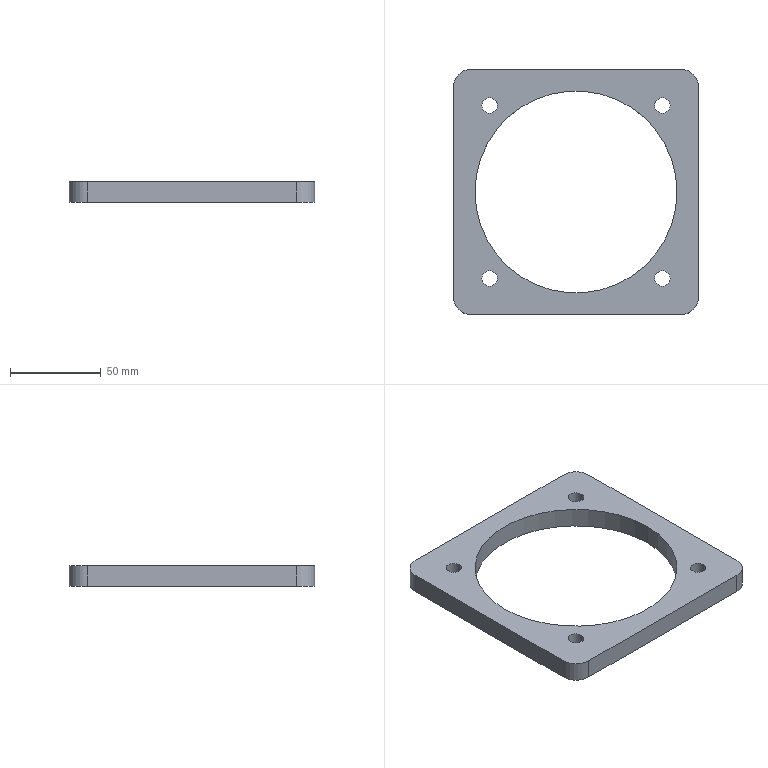Part | SolidWorks | features FlatPattern 1, HoleWzd 1, SMBaseFlange 1, SheetMetal 1 | 1 solid | 20 faces | box 135 x 135 x 11 mm | volume 90588 mm3 | cylinder 14 | plane 6 | commonest cylinder face diameters 8.5 x8 20 x4 111 x2
STEP:
#1=CARTESIAN_POINT('',(-51.75,47.5,-11.));
#2=VERTEX_POINT('',#1);
#3=CARTESIAN_POINT('',(-43.25,47.5,-11.));
#4=VERTEX_POINT('',#3);
#5=CARTESIAN_POINT('',(-47.5,47.5,-11.));
#6=DIRECTION('',(0.,0.,1.));
#7=DIRECTION('',(1.,0.,0.));
#8=AXIS2_PLACEMENT_3D('',#5,#6,#7);
#9=CIRCLE('',#8,4.25);
#10=EDGE_CURVE('',#2,#4,#9,.T.);
#11=ORIENTED_EDGE('',*,*,#10,.F.);
#12=CARTESIAN_POINT('',(-51.75,47.5,0.));
#13=VERTEX_POINT('',#12);
#14=CARTESIAN_POINT('',(-51.75,47.5,0.));
#15=DIRECTION('',(0.,0.,1.));
#16=VECTOR('',#15,1000.);
#17=LINE('',#14,#16);
#18=EDGE_CURVE('',#2,#13,#17,.T.);
#19=ORIENTED_EDGE('',*,*,#18,.T.);
#20=CARTESIAN_POINT('',(-43.25,47.5,0.));
#21=VERTEX_POINT('',#20);
#22=CARTESIAN_POINT('',(-47.5,47.5,0.));
#23=DIRECTION('',(0.,0.,1.));
#24=DIRECTION('',(1.,0.,0.));
#25=AXIS2_PLACEMENT_3D('',#22,#23,#24);
#26=CIRCLE('',#25,4.25);
#27=EDGE_CURVE('',#13,#21,#26,.T.);
#28=ORIENTED_EDGE('',*,*,#27,.T.);
#29=CARTESIAN_POINT('',(-43.25,47.5,0.));
#30=DIRECTION('',(0.,0.,1.));
#31=VECTOR('',#30,1000.);
#32=LINE('',#29,#31);
#33=EDGE_CURVE('',#4,#21,#32,.T.);
#34=ORIENTED_EDGE('',*,*,#33,.F.);
#35=EDGE_LOOP('',(#11,#19,#28,#34));
#36=FACE_OUTER_BOUND('',#35,.T.);
#37=CARTESIAN_POINT('',(-47.5,47.5,0.));
#38=DIRECTION('',(0.,0.,1.));
#39=DIRECTION('',(1.,0.,0.));
#40=AXIS2_PLACEMENT_3D('',#37,#38,#39);
#41=CYLINDRICAL_SURFACE('',#40,4.25);
#42=ADVANCED_FACE('',(#36),#41,.F.);
#43=CARTESIAN_POINT('',(43.25,47.5,-11.));
#44=VERTEX_POINT('',#43);
#45=CARTESIAN_POINT('',(51.75,47.5,-11.));
#46=VERTEX_POINT('',#45);
#47=CARTESIAN_POINT('',(47.5,47.5,-11.));
#48=DIRECTION('',(0.,0.,1.));
#49=DIRECTION('',(1.,0.,0.));
#50=AXIS2_PLACEMENT_3D('',#47,#48,#49);
#51=CIRCLE('',#50,4.25);
#52=EDGE_CURVE('',#44,#46,#51,.T.);
#53=ORIENTED_EDGE('',*,*,#52,.F.);
#54=CARTESIAN_POINT('',(43.25,47.5,0.));
#55=VERTEX_POINT('',#54);
#56=CARTESIAN_POINT('',(43.25,47.5,0.));
#57=DIRECTION('',(0.,0.,1.));
#58=VECTOR('',#57,1000.);
#59=LINE('',#56,#58);
#60=EDGE_CURVE('',#44,#55,#59,.T.);
#61=ORIENTED_EDGE('',*,*,#60,.T.);
#62=CARTESIAN_POINT('',(51.75,47.5,0.));
#63=VERTEX_POINT('',#62);
#64=CARTESIAN_POINT('',(47.5,47.5,0.));
#65=DIRECTION('',(0.,0.,1.));
#66=DIRECTION('',(1.,0.,0.));
#67=AXIS2_PLACEMENT_3D('',#64,#65,#66);
#68=CIRCLE('',#67,4.25);
#69=EDGE_CURVE('',#55,#63,#68,.T.);
#70=ORIENTED_EDGE('',*,*,#69,.T.);
#71=CARTESIAN_POINT('',(51.75,47.5,0.));
#72=DIRECTION('',(0.,0.,1.));
#73=VECTOR('',#72,1000.);
#74=LINE('',#71,#73);
#75=EDGE_CURVE('',#46,#63,#74,.T.);
#76=ORIENTED_EDGE('',*,*,#75,.F.);
#77=EDGE_LOOP('',(#53,#61,#70,#76));
#78=FACE_OUTER_BOUND('',#77,.T.);
#79=CARTESIAN_POINT('',(47.5,47.5,0.));
#80=DIRECTION('',(0.,0.,1.));
#81=DIRECTION('',(1.,0.,0.));
#82=AXIS2_PLACEMENT_3D('',#79,#80,#81);
#83=CYLINDRICAL_SURFACE('',#82,4.25);
#84=ADVANCED_FACE('',(#78),#83,.F.);
#85=CARTESIAN_POINT('',(43.25,-47.5,-11.));
#86=VERTEX_POINT('',#85);
#87=CARTESIAN_POINT('',(51.75,-47.5,-11.));
#88=VERTEX_POINT('',#87);
#89=CARTESIAN_POINT('',(47.5,-47.5,-11.));
#90=DIRECTION('',(0.,0.,1.));
#91=DIRECTION('',(1.,0.,0.));
#92=AXIS2_PLACEMENT_3D('',#89,#90,#91);
#93=CIRCLE('',#92,4.25);
#94=EDGE_CURVE('',#86,#88,#93,.T.);
#95=ORIENTED_EDGE('',*,*,#94,.F.);
#96=CARTESIAN_POINT('',(43.25,-47.5,0.));
#97=VERTEX_POINT('',#96);
#98=CARTESIAN_POINT('',(43.25,-47.5,0.));
#99=DIRECTION('',(0.,0.,1.));
#100=VECTOR('',#99,1000.);
#101=LINE('',#98,#100);
#102=EDGE_CURVE('',#86,#97,#101,.T.);
#103=ORIENTED_EDGE('',*,*,#102,.T.);
#104=CARTESIAN_POINT('',(51.75,-47.5,0.));
#105=VERTEX_POINT('',#104);
#106=CARTESIAN_POINT('',(47.5,-47.5,0.));
#107=DIRECTION('',(0.,0.,1.));
#108=DIRECTION('',(1.,0.,0.));
#109=AXIS2_PLACEMENT_3D('',#106,#107,#108);
#110=CIRCLE('',#109,4.25);
#111=EDGE_CURVE('',#97,#105,#110,.T.);
#112=ORIENTED_EDGE('',*,*,#111,.T.);
#113=CARTESIAN_POINT('',(51.75,-47.5,0.));
#114=DIRECTION('',(0.,0.,1.));
#115=VECTOR('',#114,1000.);
#116=LINE('',#113,#115);
#117=EDGE_CURVE('',#88,#105,#116,.T.);
#118=ORIENTED_EDGE('',*,*,#117,.F.);
#119=EDGE_LOOP('',(#95,#103,#112,#118));
#120=FACE_OUTER_BOUND('',#119,.T.);
#121=CARTESIAN_POINT('',(47.5,-47.5,0.));
#122=DIRECTION('',(0.,0.,1.));
#123=DIRECTION('',(1.,0.,0.));
#124=AXIS2_PLACEMENT_3D('',#121,#122,#123);
#125=CYLINDRICAL_SURFACE('',#124,4.25);
#126=ADVANCED_FACE('',(#120),#125,.F.);
#127=CARTESIAN_POINT('',(-51.75,-47.5,-11.));
#128=VERTEX_POINT('',#127);
#129=CARTESIAN_POINT('',(-43.25,-47.5,-11.));
#130=VERTEX_POINT('',#129);
#131=CARTESIAN_POINT('',(-47.5,-47.5,-11.));
#132=DIRECTION('',(0.,0.,1.));
#133=DIRECTION('',(1.,0.,0.));
#134=AXIS2_PLACEMENT_3D('',#131,#132,#133);
#135=CIRCLE('',#134,4.25);
#136=EDGE_CURVE('',#128,#130,#135,.T.);
#137=ORIENTED_EDGE('',*,*,#136,.F.);
#138=CARTESIAN_POINT('',(-51.75,-47.5,0.));
#139=VERTEX_POINT('',#138);
#140=CARTESIAN_POINT('',(-51.75,-47.5,0.));
#141=DIRECTION('',(0.,0.,1.));
#142=VECTOR('',#141,1000.);
#143=LINE('',#140,#142);
#144=EDGE_CURVE('',#128,#139,#143,.T.);
#145=ORIENTED_EDGE('',*,*,#144,.T.);
#146=CARTESIAN_POINT('',(-43.25,-47.5,0.));
#147=VERTEX_POINT('',#146);
#148=CARTESIAN_POINT('',(-47.5,-47.5,0.));
#149=DIRECTION('',(0.,0.,1.));
#150=DIRECTION('',(1.,0.,0.));
#151=AXIS2_PLACEMENT_3D('',#148,#149,#150);
#152=CIRCLE('',#151,4.25);
#153=EDGE_CURVE('',#139,#147,#152,.T.);
#154=ORIENTED_EDGE('',*,*,#153,.T.);
#155=CARTESIAN_POINT('',(-43.25,-47.5,0.));
#156=DIRECTION('',(0.,0.,1.));
#157=VECTOR('',#156,1000.);
#158=LINE('',#155,#157);
#159=EDGE_CURVE('',#130,#147,#158,.T.);
#160=ORIENTED_EDGE('',*,*,#159,.F.);
#161=EDGE_LOOP('',(#137,#145,#154,#160));
#162=FACE_OUTER_BOUND('',#161,.T.);
#163=CARTESIAN_POINT('',(-47.5,-47.5,0.));
#164=DIRECTION('',(0.,0.,1.));
#165=DIRECTION('',(1.,0.,0.));
#166=AXIS2_PLACEMENT_3D('',#163,#164,#165);
#167=CYLINDRICAL_SURFACE('',#166,4.25);
#168=ADVANCED_FACE('',(#162),#167,.F.);
#169=CARTESIAN_POINT('',(-55.5,0.,-11.));
#170=VERTEX_POINT('',#169);
#171=CARTESIAN_POINT('',(55.5,0.,-11.));
#172=VERTEX_POINT('',#171);
#173=CARTESIAN_POINT('',(0.,0.,-11.));
#174=DIRECTION('',(0.,0.,1.));
#175=DIRECTION('',(1.,0.,0.));
#176=AXIS2_PLACEMENT_3D('',#173,#174,#175);
#177=CIRCLE('',#176,55.5);
#178=EDGE_CURVE('',#170,#172,#177,.T.);
#179=ORIENTED_EDGE('',*,*,#178,.F.);
#180=CARTESIAN_POINT('',(-55.5,0.,0.));
#181=VERTEX_POINT('',#180);
#182=CARTESIAN_POINT('',(-55.5,0.,-11.));
#183=DIRECTION('',(0.,0.,1.));
#184=VECTOR('',#183,1000.);
#185=LINE('',#182,#184);
#186=EDGE_CURVE('',#170,#181,#185,.T.);
#187=ORIENTED_EDGE('',*,*,#186,.T.);
#188=CARTESIAN_POINT('',(55.5,0.,0.));
#189=VERTEX_POINT('',#188);
#190=CARTESIAN_POINT('',(0.,0.,0.));
#191=DIRECTION('',(0.,0.,1.));
#192=DIRECTION('',(1.,0.,0.));
#193=AXIS2_PLACEMENT_3D('',#190,#191,#192);
#194=CIRCLE('',#193,55.5);
#195=EDGE_CURVE('',#181,#189,#194,.T.);
#196=ORIENTED_EDGE('',*,*,#195,.T.);
#197=CARTESIAN_POINT('',(55.5,0.,-11.));
#198=DIRECTION('',(0.,0.,1.));
#199=VECTOR('',#198,1000.);
#200=LINE('',#197,#199);
#201=EDGE_CURVE('',#172,#189,#200,.T.);
#202=ORIENTED_EDGE('',*,*,#201,.F.);
#203=EDGE_LOOP('',(#179,#187,#196,#202));
#204=FACE_OUTER_BOUND('',#203,.T.);
#205=CARTESIAN_POINT('',(0.,0.,-11.));
#206=DIRECTION('',(0.,0.,1.));
#207=DIRECTION('',(1.,0.,0.));
#208=AXIS2_PLACEMENT_3D('',#205,#206,#207);
#209=CYLINDRICAL_SURFACE('',#208,55.5);
#210=ADVANCED_FACE('',(#204),#209,.F.);
#211=CARTESIAN_POINT('',(-67.5,-57.5,0.));
#212=VERTEX_POINT('',#211);
#213=CARTESIAN_POINT('',(-57.5,-67.5,0.));
#214=VERTEX_POINT('',#213);
#215=CARTESIAN_POINT('',(-57.5,-57.5,0.));
#216=DIRECTION('',(0.,0.,1.));
#217=DIRECTION('',(1.,0.,0.));
#218=AXIS2_PLACEMENT_3D('',#215,#216,#217);
#219=CIRCLE('',#218,10.);
#220=EDGE_CURVE('',#212,#214,#219,.T.);
#221=ORIENTED_EDGE('',*,*,#220,.F.);
#222=CARTESIAN_POINT('',(-67.5,-57.5,-11.));
#223=VERTEX_POINT('',#222);
#224=CARTESIAN_POINT('',(-67.5,-57.5,-11.));
#225=DIRECTION('',(0.,0.,1.));
#226=VECTOR('',#225,1000.);
#227=LINE('',#224,#226);
#228=EDGE_CURVE('',#223,#212,#227,.T.);
#229=ORIENTED_EDGE('',*,*,#228,.F.);
#230=CARTESIAN_POINT('',(-57.5,-67.5,-11.));
#231=VERTEX_POINT('',#230);
#232=CARTESIAN_POINT('',(-57.5,-57.5,-11.));
#233=DIRECTION('',(0.,0.,1.));
#234=DIRECTION('',(1.,0.,0.));
#235=AXIS2_PLACEMENT_3D('',#232,#233,#234);
#236=CIRCLE('',#235,10.);
#237=EDGE_CURVE('',#223,#231,#236,.T.);
#238=ORIENTED_EDGE('',*,*,#237,.T.);
#239=CARTESIAN_POINT('',(-57.5,-67.5,-11.));
#240=DIRECTION('',(0.,0.,1.));
#241=VECTOR('',#240,1000.);
#242=LINE('',#239,#241);
#243=EDGE_CURVE('',#231,#214,#242,.T.);
#244=ORIENTED_EDGE('',*,*,#243,.T.);
#245=EDGE_LOOP('',(#221,#229,#238,#244));
#246=FACE_OUTER_BOUND('',#245,.T.);
#247=CARTESIAN_POINT('',(-57.5,-57.5,-11.));
#248=DIRECTION('',(0.,0.,1.));
#249=DIRECTION('',(1.,0.,0.));
#250=AXIS2_PLACEMENT_3D('',#247,#248,#249);
#251=CYLINDRICAL_SURFACE('',#250,10.);
#252=ADVANCED_FACE('',(#246),#251,.T.);
#253=CARTESIAN_POINT('',(-67.5,57.5,0.));
#254=VERTEX_POINT('',#253);
#255=CARTESIAN_POINT('',(-67.5,57.5,0.));
#256=DIRECTION('',(0.,-1.,0.));
#257=VECTOR('',#256,1000.);
#258=LINE('',#255,#257);
#259=EDGE_CURVE('',#254,#212,#258,.T.);
#260=ORIENTED_EDGE('',*,*,#259,.F.);
#261=CARTESIAN_POINT('',(-67.5,57.5,-11.));
#262=VERTEX_POINT('',#261);
#263=CARTESIAN_POINT('',(-67.5,57.5,-11.));
#264=DIRECTION('',(0.,0.,1.));
#265=VECTOR('',#264,1000.);
#266=LINE('',#263,#265);
#267=EDGE_CURVE('',#262,#254,#266,.T.);
#268=ORIENTED_EDGE('',*,*,#267,.F.);
#269=CARTESIAN_POINT('',(-67.5,57.5,-11.));
#270=DIRECTION('',(0.,-1.,0.));
#271=VECTOR('',#270,1000.);
#272=LINE('',#269,#271);
#273=EDGE_CURVE('',#262,#223,#272,.T.);
#274=ORIENTED_EDGE('',*,*,#273,.T.);
#275=ORIENTED_EDGE('',*,*,#228,.T.);
#276=EDGE_LOOP('',(#260,#268,#274,#275));
#277=FACE_OUTER_BOUND('',#276,.T.);
#278=CARTESIAN_POINT('',(-67.5,57.5,-11.));
#279=DIRECTION('',(-1.,0.,0.));
#280=DIRECTION('',(0.,-1.,0.));
#281=AXIS2_PLACEMENT_3D('',#278,#279,#280);
#282=PLANE('',#281);
#283=ADVANCED_FACE('',(#277),#282,.T.);
#284=CARTESIAN_POINT('',(-57.5,67.5,0.));
#285=VERTEX_POINT('',#284);
#286=CARTESIAN_POINT('',(-57.5,57.5,0.));
#287=DIRECTION('',(0.,0.,1.));
#288=DIRECTION('',(1.,0.,0.));
#289=AXIS2_PLACEMENT_3D('',#286,#287,#288);
#290=CIRCLE('',#289,10.);
#291=EDGE_CURVE('',#285,#254,#290,.T.);
#292=ORIENTED_EDGE('',*,*,#291,.F.);
#293=CARTESIAN_POINT('',(-57.5,67.5,-11.));
#294=VERTEX_POINT('',#293);
#295=CARTESIAN_POINT('',(-57.5,67.5,-11.));
#296=DIRECTION('',(0.,0.,1.));
#297=VECTOR('',#296,1000.);
#298=LINE('',#295,#297);
#299=EDGE_CURVE('',#294,#285,#298,.T.);
#300=ORIENTED_EDGE('',*,*,#299,.F.);
#301=CARTESIAN_POINT('',(-57.5,57.5,-11.));
#302=DIRECTION('',(0.,0.,1.));
#303=DIRECTION('',(1.,0.,0.));
#304=AXIS2_PLACEMENT_3D('',#301,#302,#303);
#305=CIRCLE('',#304,10.);
#306=EDGE_CURVE('',#294,#262,#305,.T.);
#307=ORIENTED_EDGE('',*,*,#306,.T.);
#308=ORIENTED_EDGE('',*,*,#267,.T.);
#309=EDGE_LOOP('',(#292,#300,#307,#308));
#310=FACE_OUTER_BOUND('',#309,.T.);
#311=CARTESIAN_POINT('',(-57.5,57.5,-11.));
#312=DIRECTION('',(0.,0.,1.));
#313=DIRECTION('',(1.,0.,0.));
#314=AXIS2_PLACEMENT_3D('',#311,#312,#313);
#315=CYLINDRICAL_SURFACE('',#314,10.);
#316=ADVANCED_FACE('',(#310),#315,.T.);
#317=CARTESIAN_POINT('',(57.5,67.5,0.));
#318=VERTEX_POINT('',#317);
#319=CARTESIAN_POINT('',(-57.5,67.5,0.));
#320=DIRECTION('',(-1.,0.,0.));
#321=VECTOR('',#320,1000.);
#322=LINE('',#319,#321);
#323=EDGE_CURVE('',#318,#285,#322,.T.);
#324=ORIENTED_EDGE('',*,*,#323,.F.);
#325=CARTESIAN_POINT('',(57.5,67.5,-11.));
#326=VERTEX_POINT('',#325);
#327=CARTESIAN_POINT('',(57.5,67.5,-11.));
#328=DIRECTION('',(0.,0.,1.));
#329=VECTOR('',#328,1000.);
#330=LINE('',#327,#329);
#331=EDGE_CURVE('',#326,#318,#330,.T.);
#332=ORIENTED_EDGE('',*,*,#331,.F.);
#333=CARTESIAN_POINT('',(-57.5,67.5,-11.));
#334=DIRECTION('',(-1.,0.,0.));
#335=VECTOR('',#334,1000.);
#336=LINE('',#333,#335);
#337=EDGE_CURVE('',#326,#294,#336,.T.);
#338=ORIENTED_EDGE('',*,*,#337,.T.);
#339=ORIENTED_EDGE('',*,*,#299,.T.);
#340=EDGE_LOOP('',(#324,#332,#338,#339));
#341=FACE_OUTER_BOUND('',#340,.T.);
#342=CARTESIAN_POINT('',(-57.5,67.5,-11.));
#343=DIRECTION('',(0.,1.,0.));
#344=DIRECTION('',(0.,0.,1.));
#345=AXIS2_PLACEMENT_3D('',#342,#343,#344);
#346=PLANE('',#345);
#347=ADVANCED_FACE('',(#341),#346,.T.);
#348=CARTESIAN_POINT('',(67.5,57.5,0.));
#349=VERTEX_POINT('',#348);
#350=CARTESIAN_POINT('',(57.5,57.5,0.));
#351=DIRECTION('',(0.,0.,1.));
#352=DIRECTION('',(-1.,0.,0.));
#353=AXIS2_PLACEMENT_3D('',#350,#351,#352);
#354=CIRCLE('',#353,10.);
#355=EDGE_CURVE('',#349,#318,#354,.T.);
#356=ORIENTED_EDGE('',*,*,#355,.F.);
#357=CARTESIAN_POINT('',(67.5,57.5,-11.));
#358=VERTEX_POINT('',#357);
#359=CARTESIAN_POINT('',(67.5,57.5,-11.));
#360=DIRECTION('',(0.,0.,1.));
#361=VECTOR('',#360,1000.);
#362=LINE('',#359,#361);
#363=EDGE_CURVE('',#358,#349,#362,.T.);
#364=ORIENTED_EDGE('',*,*,#363,.F.);
#365=CARTESIAN_POINT('',(57.5,57.5,-11.));
#366=DIRECTION('',(0.,0.,1.));
#367=DIRECTION('',(-1.,0.,0.));
#368=AXIS2_PLACEMENT_3D('',#365,#366,#367);
#369=CIRCLE('',#368,10.);
#370=EDGE_CURVE('',#358,#326,#369,.T.);
#371=ORIENTED_EDGE('',*,*,#370,.T.);
#372=ORIENTED_EDGE('',*,*,#331,.T.);
#373=EDGE_LOOP('',(#356,#364,#371,#372));
#374=FACE_OUTER_BOUND('',#373,.T.);
#375=CARTESIAN_POINT('',(57.5,57.5,-11.));
#376=DIRECTION('',(0.,0.,1.));
#377=DIRECTION('',(1.,0.,0.));
#378=AXIS2_PLACEMENT_3D('',#375,#376,#377);
#379=CYLINDRICAL_SURFACE('',#378,10.);
#380=ADVANCED_FACE('',(#374),#379,.T.);
#381=CARTESIAN_POINT('',(67.5,-57.5,0.));
#382=VERTEX_POINT('',#381);
#383=CARTESIAN_POINT('',(67.5,57.5,0.));
#384=DIRECTION('',(0.,1.,0.));
#385=VECTOR('',#384,1000.);
#386=LINE('',#383,#385);
#387=EDGE_CURVE('',#382,#349,#386,.T.);
#388=ORIENTED_EDGE('',*,*,#387,.F.);
#389=CARTESIAN_POINT('',(67.5,-57.5,-11.));
#390=VERTEX_POINT('',#389);
#391=CARTESIAN_POINT('',(67.5,-57.5,-11.));
#392=DIRECTION('',(0.,0.,1.));
#393=VECTOR('',#392,1000.);
#394=LINE('',#391,#393);
#395=EDGE_CURVE('',#390,#382,#394,.T.);
#396=ORIENTED_EDGE('',*,*,#395,.F.);
#397=CARTESIAN_POINT('',(67.5,57.5,-11.));
#398=DIRECTION('',(0.,1.,0.));
#399=VECTOR('',#398,1000.);
#400=LINE('',#397,#399);
#401=EDGE_CURVE('',#390,#358,#400,.T.);
#402=ORIENTED_EDGE('',*,*,#401,.T.);
#403=ORIENTED_EDGE('',*,*,#363,.T.);
#404=EDGE_LOOP('',(#388,#396,#402,#403));
#405=FACE_OUTER_BOUND('',#404,.T.);
#406=CARTESIAN_POINT('',(67.5,57.5,-11.));
#407=DIRECTION('',(1.,0.,0.));
#408=DIRECTION('',(0.,1.,0.));
#409=AXIS2_PLACEMENT_3D('',#406,#407,#408);
#410=PLANE('',#409);
#411=ADVANCED_FACE('',(#405),#410,.T.);
#412=CARTESIAN_POINT('',(57.5,-67.5,0.));
#413=VERTEX_POINT('',#412);
#414=CARTESIAN_POINT('',(57.5,-57.5,0.));
#415=DIRECTION('',(0.,0.,1.));
#416=DIRECTION('',(1.,0.,0.));
#417=AXIS2_PLACEMENT_3D('',#414,#415,#416);
#418=CIRCLE('',#417,10.);
#419=EDGE_CURVE('',#413,#382,#418,.T.);
#420=ORIENTED_EDGE('',*,*,#419,.F.);
#421=CARTESIAN_POINT('',(57.5,-67.5,-11.));
#422=VERTEX_POINT('',#421);
#423=CARTESIAN_POINT('',(57.5,-67.5,-11.));
#424=DIRECTION('',(0.,0.,1.));
#425=VECTOR('',#424,1000.);
#426=LINE('',#423,#425);
#427=EDGE_CURVE('',#422,#413,#426,.T.);
#428=ORIENTED_EDGE('',*,*,#427,.F.);
#429=CARTESIAN_POINT('',(57.5,-57.5,-11.));
#430=DIRECTION('',(0.,0.,1.));
#431=DIRECTION('',(1.,0.,0.));
#432=AXIS2_PLACEMENT_3D('',#429,#430,#431);
#433=CIRCLE('',#432,10.);
#434=EDGE_CURVE('',#422,#390,#433,.T.);
#435=ORIENTED_EDGE('',*,*,#434,.T.);
#436=ORIENTED_EDGE('',*,*,#395,.T.);
#437=EDGE_LOOP('',(#420,#428,#435,#436));
#438=FACE_OUTER_BOUND('',#437,.T.);
#439=CARTESIAN_POINT('',(57.5,-57.5,-11.));
#440=DIRECTION('',(0.,0.,1.));
#441=DIRECTION('',(1.,0.,0.));
#442=AXIS2_PLACEMENT_3D('',#439,#440,#441);
#443=CYLINDRICAL_SURFACE('',#442,10.);
#444=ADVANCED_FACE('',(#438),#443,.T.);
#445=CARTESIAN_POINT('',(-57.5,-67.5,0.));
#446=DIRECTION('',(1.,0.,0.));
#447=VECTOR('',#446,1000.);
#448=LINE('',#445,#447);
#449=EDGE_CURVE('',#214,#413,#448,.T.);
#450=ORIENTED_EDGE('',*,*,#449,.F.);
#451=ORIENTED_EDGE('',*,*,#243,.F.);
#452=CARTESIAN_POINT('',(-57.5,-67.5,-11.));
#453=DIRECTION('',(1.,0.,0.));
#454=VECTOR('',#453,1000.);
#455=LINE('',#452,#454);
#456=EDGE_CURVE('',#231,#422,#455,.T.);
#457=ORIENTED_EDGE('',*,*,#456,.T.);
#458=ORIENTED_EDGE('',*,*,#427,.T.);
#459=EDGE_LOOP('',(#450,#451,#457,#458));
#460=FACE_OUTER_BOUND('',#459,.T.);
#461=CARTESIAN_POINT('',(-57.5,-67.5,-11.));
#462=DIRECTION('',(0.,-1.,0.));
#463=DIRECTION('',(0.,0.,-1.));
#464=AXIS2_PLACEMENT_3D('',#461,#462,#463);
#465=PLANE('',#464);
#466=ADVANCED_FACE('',(#460),#465,.T.);
#467=CARTESIAN_POINT('',(-47.5,47.5,-11.));
#468=DIRECTION('',(0.,0.,1.));
#469=DIRECTION('',(1.,0.,0.));
#470=AXIS2_PLACEMENT_3D('',#467,#468,#469);
#471=CIRCLE('',#470,4.25);
#472=EDGE_CURVE('',#4,#2,#471,.T.);
#473=ORIENTED_EDGE('',*,*,#472,.T.);
#474=ORIENTED_EDGE('',*,*,#10,.T.);
#475=EDGE_LOOP('',(#473,#474));
#476=FACE_BOUND('',#475,.T.);
#477=CARTESIAN_POINT('',(47.5,47.5,-11.));
#478=DIRECTION('',(0.,0.,1.));
#479=DIRECTION('',(1.,0.,0.));
#480=AXIS2_PLACEMENT_3D('',#477,#478,#479);
#481=CIRCLE('',#480,4.25);
#482=EDGE_CURVE('',#46,#44,#481,.T.);
#483=ORIENTED_EDGE('',*,*,#482,.T.);
#484=ORIENTED_EDGE('',*,*,#52,.T.);
#485=EDGE_LOOP('',(#483,#484));
#486=FACE_BOUND('',#485,.T.);
#487=CARTESIAN_POINT('',(47.5,-47.5,-11.));
#488=DIRECTION('',(0.,0.,1.));
#489=DIRECTION('',(1.,0.,0.));
#490=AXIS2_PLACEMENT_3D('',#487,#488,#489);
#491=CIRCLE('',#490,4.25);
#492=EDGE_CURVE('',#88,#86,#491,.T.);
#493=ORIENTED_EDGE('',*,*,#492,.T.);
#494=ORIENTED_EDGE('',*,*,#94,.T.);
#495=EDGE_LOOP('',(#493,#494));
#496=FACE_BOUND('',#495,.T.);
#497=CARTESIAN_POINT('',(-47.5,-47.5,-11.));
#498=DIRECTION('',(0.,0.,1.));
#499=DIRECTION('',(1.,0.,0.));
#500=AXIS2_PLACEMENT_3D('',#497,#498,#499);
#501=CIRCLE('',#500,4.25);
#502=EDGE_CURVE('',#130,#128,#501,.T.);
#503=ORIENTED_EDGE('',*,*,#502,.T.);
#504=ORIENTED_EDGE('',*,*,#136,.T.);
#505=EDGE_LOOP('',(#503,#504));
#506=FACE_BOUND('',#505,.T.);
#507=CARTESIAN_POINT('',(0.,0.,-11.));
#508=DIRECTION('',(0.,0.,1.));
#509=DIRECTION('',(1.,0.,0.));
#510=AXIS2_PLACEMENT_3D('',#507,#508,#509);
#511=CIRCLE('',#510,55.5);
#512=EDGE_CURVE('',#172,#170,#511,.T.);
#513=ORIENTED_EDGE('',*,*,#512,.T.);
#514=ORIENTED_EDGE('',*,*,#178,.T.);
#515=EDGE_LOOP('',(#513,#514));
#516=FACE_BOUND('',#515,.T.);
#517=ORIENTED_EDGE('',*,*,#237,.F.);
#518=ORIENTED_EDGE('',*,*,#273,.F.);
#519=ORIENTED_EDGE('',*,*,#306,.F.);
#520=ORIENTED_EDGE('',*,*,#337,.F.);
#521=ORIENTED_EDGE('',*,*,#370,.F.);
#522=ORIENTED_EDGE('',*,*,#401,.F.);
#523=ORIENTED_EDGE('',*,*,#434,.F.);
#524=ORIENTED_EDGE('',*,*,#456,.F.);
#525=EDGE_LOOP('',(#517,#518,#519,#520,#521,#522,#523,#524));
#526=FACE_OUTER_BOUND('',#525,.T.);
#527=CARTESIAN_POINT('',(-57.5,-57.5,-11.));
#528=DIRECTION('',(0.,0.,1.));
#529=DIRECTION('',(1.,0.,0.));
#530=AXIS2_PLACEMENT_3D('',#527,#528,#529);
#531=PLANE('',#530);
#532=ADVANCED_FACE('',(#476,#486,#496,#506,#516,#526),#531,.F.);
#533=CARTESIAN_POINT('',(-47.5,47.5,0.));
#534=DIRECTION('',(0.,0.,1.));
#535=DIRECTION('',(1.,0.,0.));
#536=AXIS2_PLACEMENT_3D('',#533,#534,#535);
#537=CIRCLE('',#536,4.25);
#538=EDGE_CURVE('',#21,#13,#537,.T.);
#539=ORIENTED_EDGE('',*,*,#538,.F.);
#540=ORIENTED_EDGE('',*,*,#27,.F.);
#541=EDGE_LOOP('',(#539,#540));
#542=FACE_BOUND('',#541,.T.);
#543=CARTESIAN_POINT('',(47.5,47.5,0.));
#544=DIRECTION('',(0.,0.,1.));
#545=DIRECTION('',(1.,0.,0.));
#546=AXIS2_PLACEMENT_3D('',#543,#544,#545);
#547=CIRCLE('',#546,4.25);
#548=EDGE_CURVE('',#63,#55,#547,.T.);
#549=ORIENTED_EDGE('',*,*,#548,.F.);
#550=ORIENTED_EDGE('',*,*,#69,.F.);
#551=EDGE_LOOP('',(#549,#550));
#552=FACE_BOUND('',#551,.T.);
#553=CARTESIAN_POINT('',(47.5,-47.5,0.));
#554=DIRECTION('',(0.,0.,1.));
#555=DIRECTION('',(1.,0.,0.));
#556=AXIS2_PLACEMENT_3D('',#553,#554,#555);
#557=CIRCLE('',#556,4.25);
#558=EDGE_CURVE('',#105,#97,#557,.T.);
#559=ORIENTED_EDGE('',*,*,#558,.F.);
#560=ORIENTED_EDGE('',*,*,#111,.F.);
#561=EDGE_LOOP('',(#559,#560));
#562=FACE_BOUND('',#561,.T.);
#563=CARTESIAN_POINT('',(-47.5,-47.5,0.));
#564=DIRECTION('',(0.,0.,1.));
#565=DIRECTION('',(1.,0.,0.));
#566=AXIS2_PLACEMENT_3D('',#563,#564,#565);
#567=CIRCLE('',#566,4.25);
#568=EDGE_CURVE('',#147,#139,#567,.T.);
#569=ORIENTED_EDGE('',*,*,#568,.F.);
#570=ORIENTED_EDGE('',*,*,#153,.F.);
#571=EDGE_LOOP('',(#569,#570));
#572=FACE_BOUND('',#571,.T.);
#573=CARTESIAN_POINT('',(0.,0.,0.));
#574=DIRECTION('',(0.,0.,1.));
#575=DIRECTION('',(1.,0.,0.));
#576=AXIS2_PLACEMENT_3D('',#573,#574,#575);
#577=CIRCLE('',#576,55.5);
#578=EDGE_CURVE('',#189,#181,#577,.T.);
#579=ORIENTED_EDGE('',*,*,#578,.F.);
#580=ORIENTED_EDGE('',*,*,#195,.F.);
#581=EDGE_LOOP('',(#579,#580));
#582=FACE_BOUND('',#581,.T.);
#583=ORIENTED_EDGE('',*,*,#220,.T.);
#584=ORIENTED_EDGE('',*,*,#449,.T.);
#585=ORIENTED_EDGE('',*,*,#419,.T.);
#586=ORIENTED_EDGE('',*,*,#387,.T.);
#587=ORIENTED_EDGE('',*,*,#355,.T.);
#588=ORIENTED_EDGE('',*,*,#323,.T.);
#589=ORIENTED_EDGE('',*,*,#291,.T.);
#590=ORIENTED_EDGE('',*,*,#259,.T.);
#591=EDGE_LOOP('',(#583,#584,#585,#586,#587,#588,#589,#590));
#592=FACE_OUTER_BOUND('',#591,.T.);
#593=CARTESIAN_POINT('',(-57.5,-57.5,0.));
#594=DIRECTION('',(0.,0.,1.));
#595=DIRECTION('',(1.,0.,0.));
#596=AXIS2_PLACEMENT_3D('',#593,#594,#595);
#597=PLANE('',#596);
#598=ADVANCED_FACE('',(#542,#552,#562,#572,#582,#592),#597,.T.);
#599=ORIENTED_EDGE('',*,*,#186,.F.);
#600=ORIENTED_EDGE('',*,*,#512,.F.);
#601=ORIENTED_EDGE('',*,*,#201,.T.);
#602=ORIENTED_EDGE('',*,*,#578,.T.);
#603=EDGE_LOOP('',(#599,#600,#601,#602));
#604=FACE_OUTER_BOUND('',#603,.T.);
#605=CARTESIAN_POINT('',(0.,0.,-11.));
#606=DIRECTION('',(0.,0.,1.));
#607=DIRECTION('',(1.,0.,0.));
#608=AXIS2_PLACEMENT_3D('',#605,#606,#607);
#609=CYLINDRICAL_SURFACE('',#608,55.5);
#610=ADVANCED_FACE('',(#604),#609,.F.);
#611=ORIENTED_EDGE('',*,*,#144,.F.);
#612=ORIENTED_EDGE('',*,*,#502,.F.);
#613=ORIENTED_EDGE('',*,*,#159,.T.);
#614=ORIENTED_EDGE('',*,*,#568,.T.);
#615=EDGE_LOOP('',(#611,#612,#613,#614));
#616=FACE_OUTER_BOUND('',#615,.T.);
#617=CARTESIAN_POINT('',(-47.5,-47.5,0.));
#618=DIRECTION('',(0.,0.,1.));
#619=DIRECTION('',(1.,0.,0.));
#620=AXIS2_PLACEMENT_3D('',#617,#618,#619);
#621=CYLINDRICAL_SURFACE('',#620,4.25);
#622=ADVANCED_FACE('',(#616),#621,.F.);
#623=ORIENTED_EDGE('',*,*,#102,.F.);
#624=ORIENTED_EDGE('',*,*,#492,.F.);
#625=ORIENTED_EDGE('',*,*,#117,.T.);
#626=ORIENTED_EDGE('',*,*,#558,.T.);
#627=EDGE_LOOP('',(#623,#624,#625,#626));
#628=FACE_OUTER_BOUND('',#627,.T.);
#629=CARTESIAN_POINT('',(47.5,-47.5,0.));
#630=DIRECTION('',(0.,0.,1.));
#631=DIRECTION('',(1.,0.,0.));
#632=AXIS2_PLACEMENT_3D('',#629,#630,#631);
#633=CYLINDRICAL_SURFACE('',#632,4.25);
#634=ADVANCED_FACE('',(#628),#633,.F.);
#635=ORIENTED_EDGE('',*,*,#60,.F.);
#636=ORIENTED_EDGE('',*,*,#482,.F.);
#637=ORIENTED_EDGE('',*,*,#75,.T.);
#638=ORIENTED_EDGE('',*,*,#548,.T.);
#639=EDGE_LOOP('',(#635,#636,#637,#638));
#640=FACE_OUTER_BOUND('',#639,.T.);
#641=CARTESIAN_POINT('',(47.5,47.5,0.));
#642=DIRECTION('',(0.,0.,1.));
#643=DIRECTION('',(1.,0.,0.));
#644=AXIS2_PLACEMENT_3D('',#641,#642,#643);
#645=CYLINDRICAL_SURFACE('',#644,4.25);
#646=ADVANCED_FACE('',(#640),#645,.F.);
#647=ORIENTED_EDGE('',*,*,#18,.F.);
#648=ORIENTED_EDGE('',*,*,#472,.F.);
#649=ORIENTED_EDGE('',*,*,#33,.T.);
#650=ORIENTED_EDGE('',*,*,#538,.T.);
#651=EDGE_LOOP('',(#647,#648,#649,#650));
#652=FACE_OUTER_BOUND('',#651,.T.);
#653=CARTESIAN_POINT('',(-47.5,47.5,0.));
#654=DIRECTION('',(0.,0.,1.));
#655=DIRECTION('',(1.,0.,0.));
#656=AXIS2_PLACEMENT_3D('',#653,#654,#655);
#657=CYLINDRICAL_SURFACE('',#656,4.25);
#658=ADVANCED_FACE('',(#652),#657,.F.);
#659=CLOSED_SHELL('',(#42,#84,#126,#168,#210,#252,#283,#316,#347,#380,#411,#444,#466,#532,#598,#610,#622,#634,#646,#658));
#660=MANIFOLD_SOLID_BREP('',#659);
#661=CARTESIAN_POINT('',(0.,0.,0.));
#662=DIRECTION('',(0.,0.,1.));
#663=DIRECTION('',(1.,0.,0.));
#664=AXIS2_PLACEMENT_3D('',#661,#662,#663);
#665=(LENGTH_UNIT()NAMED_UNIT(*)SI_UNIT(.MILLI.,.METRE.));
#666=UNCERTAINTY_MEASURE_WITH_UNIT(LENGTH_MEASURE(0.00001),#665,'','');
#667=(NAMED_UNIT(*)PLANE_ANGLE_UNIT()SI_UNIT($,.RADIAN.));
#668=(NAMED_UNIT(*)SI_UNIT($,.STERADIAN.)SOLID_ANGLE_UNIT());
#669=(GEOMETRIC_REPRESENTATION_CONTEXT(3)GLOBAL_UNCERTAINTY_ASSIGNED_CONTEXT((#666))GLOBAL_UNIT_ASSIGNED_CONTEXT((#665,#667,#668))REPRESENTATION_CONTEXT('',''));
#670=ADVANCED_BREP_SHAPE_REPRESENTATION('',(#660,#664),#669);